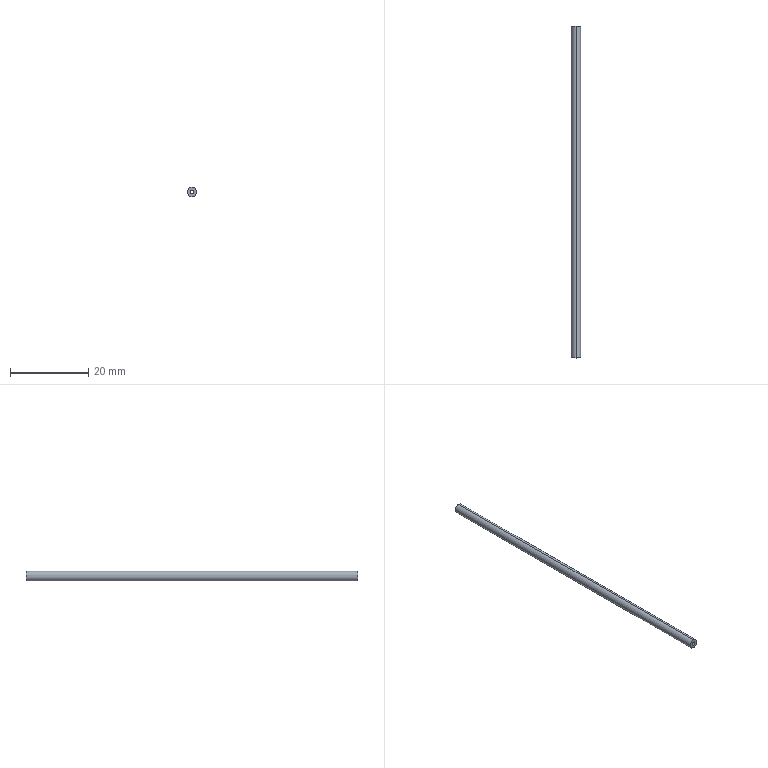Part | SolidWorks | features Revolution 1 | 1 solid | 6 faces | box 2.4 x 85 x 2.4 mm | volume 317.772 mm3 | cylinder 4 | plane 2 | commonest cylinder face diameters 1 x2 2.4 x2
STEP:
#1=CARTESIAN_POINT('',(0.,85.,-1.2));
#2=VERTEX_POINT('',#1);
#3=CARTESIAN_POINT('',(0.,85.,1.2));
#4=VERTEX_POINT('',#3);
#5=CARTESIAN_POINT('',(0.,85.,0.));
#6=DIRECTION('',(0.,-1.,0.));
#7=DIRECTION('',(0.,0.,-1.));
#8=AXIS2_PLACEMENT_3D('',#5,#6,#7);
#9=CIRCLE('',#8,1.2);
#10=EDGE_CURVE('',#2,#4,#9,.T.);
#11=ORIENTED_EDGE('',*,*,#10,.T.);
#12=CARTESIAN_POINT('',(0.,0.,1.2));
#13=VERTEX_POINT('',#12);
#14=CARTESIAN_POINT('',(0.,-6.442,1.2));
#15=DIRECTION('',(0.,-1.,0.));
#16=VECTOR('',#15,1000.);
#17=LINE('',#14,#16);
#18=EDGE_CURVE('',#4,#13,#17,.T.);
#19=ORIENTED_EDGE('',*,*,#18,.T.);
#20=CARTESIAN_POINT('',(0.,0.,-1.2));
#21=VERTEX_POINT('',#20);
#22=CARTESIAN_POINT('',(0.,0.,0.));
#23=DIRECTION('',(0.,-1.,0.));
#24=DIRECTION('',(0.,0.,-1.));
#25=AXIS2_PLACEMENT_3D('',#22,#23,#24);
#26=CIRCLE('',#25,1.2);
#27=EDGE_CURVE('',#21,#13,#26,.T.);
#28=ORIENTED_EDGE('',*,*,#27,.F.);
#29=CARTESIAN_POINT('',(0.,-6.442,-1.2));
#30=DIRECTION('',(0.,-1.,0.));
#31=VECTOR('',#30,1000.);
#32=LINE('',#29,#31);
#33=EDGE_CURVE('',#2,#21,#32,.T.);
#34=ORIENTED_EDGE('',*,*,#33,.F.);
#35=EDGE_LOOP('',(#11,#19,#28,#34));
#36=FACE_OUTER_BOUND('',#35,.T.);
#37=CARTESIAN_POINT('',(0.,-6.442,0.));
#38=DIRECTION('',(0.,-1.,0.));
#39=DIRECTION('',(0.,0.,-1.));
#40=AXIS2_PLACEMENT_3D('',#37,#38,#39);
#41=CYLINDRICAL_SURFACE('',#40,1.2);
#42=ADVANCED_FACE('',(#36),#41,.T.);
#43=CARTESIAN_POINT('',(0.,85.,0.5));
#44=VERTEX_POINT('',#43);
#45=CARTESIAN_POINT('',(0.,85.,-0.5));
#46=VERTEX_POINT('',#45);
#47=CARTESIAN_POINT('',(0.,85.,0.));
#48=DIRECTION('',(0.,-1.,0.));
#49=DIRECTION('',(0.,0.,-1.));
#50=AXIS2_PLACEMENT_3D('',#47,#48,#49);
#51=CIRCLE('',#50,0.5);
#52=EDGE_CURVE('',#44,#46,#51,.T.);
#53=ORIENTED_EDGE('',*,*,#52,.F.);
#54=CARTESIAN_POINT('',(0.,0.,0.5));
#55=VERTEX_POINT('',#54);
#56=CARTESIAN_POINT('',(0.,-6.442,0.5));
#57=DIRECTION('',(0.,-1.,0.));
#58=VECTOR('',#57,1000.);
#59=LINE('',#56,#58);
#60=EDGE_CURVE('',#44,#55,#59,.T.);
#61=ORIENTED_EDGE('',*,*,#60,.T.);
#62=CARTESIAN_POINT('',(0.,0.,-0.5));
#63=VERTEX_POINT('',#62);
#64=CARTESIAN_POINT('',(0.,0.,0.));
#65=DIRECTION('',(0.,-1.,0.));
#66=DIRECTION('',(0.,0.,-1.));
#67=AXIS2_PLACEMENT_3D('',#64,#65,#66);
#68=CIRCLE('',#67,0.5);
#69=EDGE_CURVE('',#55,#63,#68,.T.);
#70=ORIENTED_EDGE('',*,*,#69,.T.);
#71=CARTESIAN_POINT('',(0.,-6.442,-0.5));
#72=DIRECTION('',(0.,-1.,0.));
#73=VECTOR('',#72,1000.);
#74=LINE('',#71,#73);
#75=EDGE_CURVE('',#46,#63,#74,.T.);
#76=ORIENTED_EDGE('',*,*,#75,.F.);
#77=EDGE_LOOP('',(#53,#61,#70,#76));
#78=FACE_OUTER_BOUND('',#77,.T.);
#79=CARTESIAN_POINT('',(0.,-6.442,0.));
#80=DIRECTION('',(0.,-1.,0.));
#81=DIRECTION('',(0.,0.,-1.));
#82=AXIS2_PLACEMENT_3D('',#79,#80,#81);
#83=CYLINDRICAL_SURFACE('',#82,0.5);
#84=ADVANCED_FACE('',(#78),#83,.F.);
#85=ORIENTED_EDGE('',*,*,#60,.F.);
#86=CARTESIAN_POINT('',(0.,85.,0.));
#87=DIRECTION('',(0.,-1.,0.));
#88=DIRECTION('',(0.,0.,-1.));
#89=AXIS2_PLACEMENT_3D('',#86,#87,#88);
#90=CIRCLE('',#89,0.5);
#91=EDGE_CURVE('',#46,#44,#90,.T.);
#92=ORIENTED_EDGE('',*,*,#91,.F.);
#93=ORIENTED_EDGE('',*,*,#75,.T.);
#94=CARTESIAN_POINT('',(0.,0.,0.));
#95=DIRECTION('',(0.,-1.,0.));
#96=DIRECTION('',(0.,0.,-1.));
#97=AXIS2_PLACEMENT_3D('',#94,#95,#96);
#98=CIRCLE('',#97,0.5);
#99=EDGE_CURVE('',#63,#55,#98,.T.);
#100=ORIENTED_EDGE('',*,*,#99,.T.);
#101=EDGE_LOOP('',(#85,#92,#93,#100));
#102=FACE_OUTER_BOUND('',#101,.T.);
#103=CARTESIAN_POINT('',(0.,-6.442,0.));
#104=DIRECTION('',(0.,-1.,0.));
#105=DIRECTION('',(0.,0.,-1.));
#106=AXIS2_PLACEMENT_3D('',#103,#104,#105);
#107=CYLINDRICAL_SURFACE('',#106,0.5);
#108=ADVANCED_FACE('',(#102),#107,.F.);
#109=ORIENTED_EDGE('',*,*,#10,.F.);
#110=CARTESIAN_POINT('',(0.,85.,0.));
#111=DIRECTION('',(0.,-1.,0.));
#112=DIRECTION('',(0.,0.,-1.));
#113=AXIS2_PLACEMENT_3D('',#110,#111,#112);
#114=CIRCLE('',#113,1.2);
#115=EDGE_CURVE('',#4,#2,#114,.T.);
#116=ORIENTED_EDGE('',*,*,#115,.F.);
#117=EDGE_LOOP('',(#109,#116));
#118=FACE_OUTER_BOUND('',#117,.T.);
#119=ORIENTED_EDGE('',*,*,#91,.T.);
#120=ORIENTED_EDGE('',*,*,#52,.T.);
#121=EDGE_LOOP('',(#119,#120));
#122=FACE_BOUND('',#121,.T.);
#123=CARTESIAN_POINT('',(-0.5,85.,0.));
#124=DIRECTION('',(0.,-1.,0.));
#125=DIRECTION('',(0.,0.,-1.));
#126=AXIS2_PLACEMENT_3D('',#123,#124,#125);
#127=PLANE('',#126);
#128=ADVANCED_FACE('',(#118,#122),#127,.F.);
#129=ORIENTED_EDGE('',*,*,#18,.F.);
#130=ORIENTED_EDGE('',*,*,#115,.T.);
#131=ORIENTED_EDGE('',*,*,#33,.T.);
#132=CARTESIAN_POINT('',(0.,0.,0.));
#133=DIRECTION('',(0.,-1.,0.));
#134=DIRECTION('',(0.,0.,-1.));
#135=AXIS2_PLACEMENT_3D('',#132,#133,#134);
#136=CIRCLE('',#135,1.2);
#137=EDGE_CURVE('',#13,#21,#136,.T.);
#138=ORIENTED_EDGE('',*,*,#137,.F.);
#139=EDGE_LOOP('',(#129,#130,#131,#138));
#140=FACE_OUTER_BOUND('',#139,.T.);
#141=CARTESIAN_POINT('',(0.,-6.442,0.));
#142=DIRECTION('',(0.,-1.,0.));
#143=DIRECTION('',(0.,0.,-1.));
#144=AXIS2_PLACEMENT_3D('',#141,#142,#143);
#145=CYLINDRICAL_SURFACE('',#144,1.2);
#146=ADVANCED_FACE('',(#140),#145,.T.);
#147=ORIENTED_EDGE('',*,*,#99,.F.);
#148=ORIENTED_EDGE('',*,*,#69,.F.);
#149=EDGE_LOOP('',(#147,#148));
#150=FACE_BOUND('',#149,.T.);
#151=ORIENTED_EDGE('',*,*,#27,.T.);
#152=ORIENTED_EDGE('',*,*,#137,.T.);
#153=EDGE_LOOP('',(#151,#152));
#154=FACE_OUTER_BOUND('',#153,.T.);
#155=CARTESIAN_POINT('',(-0.5,0.,0.));
#156=DIRECTION('',(0.,1.,0.));
#157=DIRECTION('',(0.,0.,1.));
#158=AXIS2_PLACEMENT_3D('',#155,#156,#157);
#159=PLANE('',#158);
#160=ADVANCED_FACE('',(#150,#154),#159,.F.);
#161=CLOSED_SHELL('',(#42,#84,#108,#128,#146,#160));
#162=MANIFOLD_SOLID_BREP('',#161);
#163=CARTESIAN_POINT('',(0.,0.,0.));
#164=DIRECTION('',(0.,0.,1.));
#165=DIRECTION('',(1.,0.,0.));
#166=AXIS2_PLACEMENT_3D('',#163,#164,#165);
#167=(LENGTH_UNIT()NAMED_UNIT(*)SI_UNIT(.MILLI.,.METRE.));
#168=UNCERTAINTY_MEASURE_WITH_UNIT(LENGTH_MEASURE(0.00001),#167,'','');
#169=(NAMED_UNIT(*)PLANE_ANGLE_UNIT()SI_UNIT($,.RADIAN.));
#170=(NAMED_UNIT(*)SI_UNIT($,.STERADIAN.)SOLID_ANGLE_UNIT());
#171=(GEOMETRIC_REPRESENTATION_CONTEXT(3)GLOBAL_UNCERTAINTY_ASSIGNED_CONTEXT((#168))GLOBAL_UNIT_ASSIGNED_CONTEXT((#167,#169,#170))REPRESENTATION_CONTEXT('',''));
#172=ADVANCED_BREP_SHAPE_REPRESENTATION('',(#162,#166),#171);